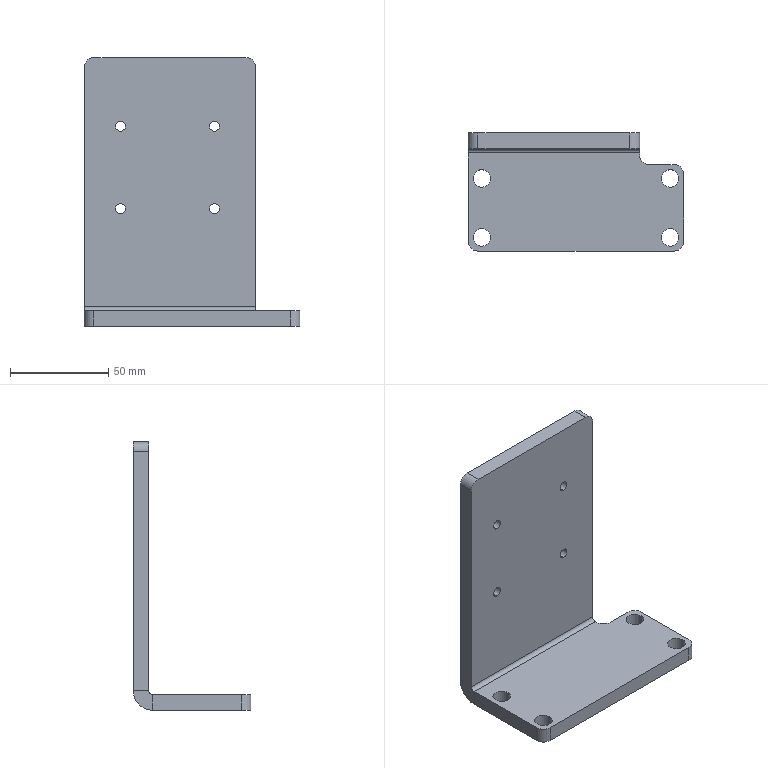Part | SolidWorks | features HoleWzd 2, EdgeFlange 1, Fillet 1, FlatPattern 1, ICE 1, SMBaseFlange 1, SheetMetal 1 | 1 solid | 38 faces | box 110 x 60 x 137 mm | volume 135582 mm3 | cylinder 24 | plane 14 | commonest cylinder face diameters 5 x8 9 x8 10 x6 4 x1 20 x1
STEP:
#1=CARTESIAN_POINT('',(107.5,7.,0.));
#2=VERTEX_POINT('',#1);
#3=CARTESIAN_POINT('',(98.5,7.,0.));
#4=VERTEX_POINT('',#3);
#5=CARTESIAN_POINT('',(103.,7.,0.));
#6=DIRECTION('',(0.,0.,-1.));
#7=DIRECTION('',(-1.,0.,0.));
#8=AXIS2_PLACEMENT_3D('',#5,#6,#7);
#9=CIRCLE('',#8,4.5);
#10=EDGE_CURVE('',#2,#4,#9,.T.);
#11=ORIENTED_EDGE('',*,*,#10,.F.);
#12=CARTESIAN_POINT('',(107.5,7.,-8.));
#13=VERTEX_POINT('',#12);
#14=CARTESIAN_POINT('',(107.5,7.,-8.));
#15=DIRECTION('',(0.,0.,-1.));
#16=VECTOR('',#15,1000.);
#17=LINE('',#14,#16);
#18=EDGE_CURVE('',#2,#13,#17,.T.);
#19=ORIENTED_EDGE('',*,*,#18,.T.);
#20=CARTESIAN_POINT('',(98.5,7.,-8.));
#21=VERTEX_POINT('',#20);
#22=CARTESIAN_POINT('',(103.,7.,-8.));
#23=DIRECTION('',(0.,0.,-1.));
#24=DIRECTION('',(-1.,0.,0.));
#25=AXIS2_PLACEMENT_3D('',#22,#23,#24);
#26=CIRCLE('',#25,4.5);
#27=EDGE_CURVE('',#13,#21,#26,.T.);
#28=ORIENTED_EDGE('',*,*,#27,.T.);
#29=CARTESIAN_POINT('',(98.5,7.,-8.));
#30=DIRECTION('',(0.,0.,-1.));
#31=VECTOR('',#30,1000.);
#32=LINE('',#29,#31);
#33=EDGE_CURVE('',#4,#21,#32,.T.);
#34=ORIENTED_EDGE('',*,*,#33,.F.);
#35=EDGE_LOOP('',(#11,#19,#28,#34));
#36=FACE_OUTER_BOUND('',#35,.T.);
#37=CARTESIAN_POINT('',(103.,7.,-8.));
#38=DIRECTION('',(0.,0.,-1.));
#39=DIRECTION('',(-1.,0.,0.));
#40=AXIS2_PLACEMENT_3D('',#37,#38,#39);
#41=CYLINDRICAL_SURFACE('',#40,4.5);
#42=ADVANCED_FACE('',(#36),#41,.F.);
#43=CARTESIAN_POINT('',(107.5,37.,0.));
#44=VERTEX_POINT('',#43);
#45=CARTESIAN_POINT('',(98.5,37.,0.));
#46=VERTEX_POINT('',#45);
#47=CARTESIAN_POINT('',(103.,37.,0.));
#48=DIRECTION('',(0.,0.,-1.));
#49=DIRECTION('',(-1.,0.,0.));
#50=AXIS2_PLACEMENT_3D('',#47,#48,#49);
#51=CIRCLE('',#50,4.5);
#52=EDGE_CURVE('',#44,#46,#51,.T.);
#53=ORIENTED_EDGE('',*,*,#52,.F.);
#54=CARTESIAN_POINT('',(107.5,37.,-8.));
#55=VERTEX_POINT('',#54);
#56=CARTESIAN_POINT('',(107.5,37.,-8.));
#57=DIRECTION('',(0.,0.,-1.));
#58=VECTOR('',#57,1000.);
#59=LINE('',#56,#58);
#60=EDGE_CURVE('',#44,#55,#59,.T.);
#61=ORIENTED_EDGE('',*,*,#60,.T.);
#62=CARTESIAN_POINT('',(98.5,37.,-8.));
#63=VERTEX_POINT('',#62);
#64=CARTESIAN_POINT('',(103.,37.,-8.));
#65=DIRECTION('',(0.,0.,-1.));
#66=DIRECTION('',(-1.,0.,0.));
#67=AXIS2_PLACEMENT_3D('',#64,#65,#66);
#68=CIRCLE('',#67,4.5);
#69=EDGE_CURVE('',#55,#63,#68,.T.);
#70=ORIENTED_EDGE('',*,*,#69,.T.);
#71=CARTESIAN_POINT('',(98.5,37.,-8.));
#72=DIRECTION('',(0.,0.,-1.));
#73=VECTOR('',#72,1000.);
#74=LINE('',#71,#73);
#75=EDGE_CURVE('',#46,#63,#74,.T.);
#76=ORIENTED_EDGE('',*,*,#75,.F.);
#77=EDGE_LOOP('',(#53,#61,#70,#76));
#78=FACE_OUTER_BOUND('',#77,.T.);
#79=CARTESIAN_POINT('',(103.,37.,-8.));
#80=DIRECTION('',(0.,0.,-1.));
#81=DIRECTION('',(-1.,0.,0.));
#82=AXIS2_PLACEMENT_3D('',#79,#80,#81);
#83=CYLINDRICAL_SURFACE('',#82,4.5);
#84=ADVANCED_FACE('',(#78),#83,.F.);
#85=CARTESIAN_POINT('',(11.5,7.,0.));
#86=VERTEX_POINT('',#85);
#87=CARTESIAN_POINT('',(2.5,7.,0.));
#88=VERTEX_POINT('',#87);
#89=CARTESIAN_POINT('',(7.,7.,0.));
#90=DIRECTION('',(0.,0.,-1.));
#91=DIRECTION('',(-1.,0.,0.));
#92=AXIS2_PLACEMENT_3D('',#89,#90,#91);
#93=CIRCLE('',#92,4.5);
#94=EDGE_CURVE('',#86,#88,#93,.T.);
#95=ORIENTED_EDGE('',*,*,#94,.F.);
#96=CARTESIAN_POINT('',(11.5,7.,-8.));
#97=VERTEX_POINT('',#96);
#98=CARTESIAN_POINT('',(11.5,7.,-8.));
#99=DIRECTION('',(0.,0.,-1.));
#100=VECTOR('',#99,1000.);
#101=LINE('',#98,#100);
#102=EDGE_CURVE('',#86,#97,#101,.T.);
#103=ORIENTED_EDGE('',*,*,#102,.T.);
#104=CARTESIAN_POINT('',(2.5,7.,-8.));
#105=VERTEX_POINT('',#104);
#106=CARTESIAN_POINT('',(7.,7.,-8.));
#107=DIRECTION('',(0.,0.,-1.));
#108=DIRECTION('',(-1.,0.,0.));
#109=AXIS2_PLACEMENT_3D('',#106,#107,#108);
#110=CIRCLE('',#109,4.5);
#111=EDGE_CURVE('',#97,#105,#110,.T.);
#112=ORIENTED_EDGE('',*,*,#111,.T.);
#113=CARTESIAN_POINT('',(2.5,7.,-8.));
#114=DIRECTION('',(0.,0.,-1.));
#115=VECTOR('',#114,1000.);
#116=LINE('',#113,#115);
#117=EDGE_CURVE('',#88,#105,#116,.T.);
#118=ORIENTED_EDGE('',*,*,#117,.F.);
#119=EDGE_LOOP('',(#95,#103,#112,#118));
#120=FACE_OUTER_BOUND('',#119,.T.);
#121=CARTESIAN_POINT('',(7.,7.,-8.));
#122=DIRECTION('',(0.,0.,-1.));
#123=DIRECTION('',(-1.,0.,0.));
#124=AXIS2_PLACEMENT_3D('',#121,#122,#123);
#125=CYLINDRICAL_SURFACE('',#124,4.5);
#126=ADVANCED_FACE('',(#120),#125,.F.);
#127=CARTESIAN_POINT('',(11.5,37.,0.));
#128=VERTEX_POINT('',#127);
#129=CARTESIAN_POINT('',(2.5,37.,0.));
#130=VERTEX_POINT('',#129);
#131=CARTESIAN_POINT('',(7.,37.,0.));
#132=DIRECTION('',(0.,0.,-1.));
#133=DIRECTION('',(-1.,0.,0.));
#134=AXIS2_PLACEMENT_3D('',#131,#132,#133);
#135=CIRCLE('',#134,4.5);
#136=EDGE_CURVE('',#128,#130,#135,.T.);
#137=ORIENTED_EDGE('',*,*,#136,.F.);
#138=CARTESIAN_POINT('',(11.5,37.,-8.));
#139=VERTEX_POINT('',#138);
#140=CARTESIAN_POINT('',(11.5,37.,-8.));
#141=DIRECTION('',(0.,0.,-1.));
#142=VECTOR('',#141,1000.);
#143=LINE('',#140,#142);
#144=EDGE_CURVE('',#128,#139,#143,.T.);
#145=ORIENTED_EDGE('',*,*,#144,.T.);
#146=CARTESIAN_POINT('',(2.5,37.,-8.));
#147=VERTEX_POINT('',#146);
#148=CARTESIAN_POINT('',(7.,37.,-8.));
#149=DIRECTION('',(0.,0.,-1.));
#150=DIRECTION('',(-1.,0.,0.));
#151=AXIS2_PLACEMENT_3D('',#148,#149,#150);
#152=CIRCLE('',#151,4.5);
#153=EDGE_CURVE('',#139,#147,#152,.T.);
#154=ORIENTED_EDGE('',*,*,#153,.T.);
#155=CARTESIAN_POINT('',(2.5,37.,-8.));
#156=DIRECTION('',(0.,0.,-1.));
#157=VECTOR('',#156,1000.);
#158=LINE('',#155,#157);
#159=EDGE_CURVE('',#130,#147,#158,.T.);
#160=ORIENTED_EDGE('',*,*,#159,.F.);
#161=EDGE_LOOP('',(#137,#145,#154,#160));
#162=FACE_OUTER_BOUND('',#161,.T.);
#163=CARTESIAN_POINT('',(7.,37.,-8.));
#164=DIRECTION('',(0.,0.,-1.));
#165=DIRECTION('',(-1.,0.,0.));
#166=AXIS2_PLACEMENT_3D('',#163,#164,#165);
#167=CYLINDRICAL_SURFACE('',#166,4.5);
#168=ADVANCED_FACE('',(#162),#167,.F.);
#169=CARTESIAN_POINT('',(18.5,52.,54.5));
#170=VERTEX_POINT('',#169);
#171=CARTESIAN_POINT('',(18.5,52.,49.5));
#172=VERTEX_POINT('',#171);
#173=CARTESIAN_POINT('',(18.5,52.,52.));
#174=DIRECTION('',(0.,-1.,0.));
#175=DIRECTION('',(0.,0.,-1.));
#176=AXIS2_PLACEMENT_3D('',#173,#174,#175);
#177=CIRCLE('',#176,2.5);
#178=EDGE_CURVE('',#170,#172,#177,.T.);
#179=ORIENTED_EDGE('',*,*,#178,.T.);
#180=CARTESIAN_POINT('',(18.5,60.,49.5));
#181=VERTEX_POINT('',#180);
#182=CARTESIAN_POINT('',(18.5,60.,49.5));
#183=DIRECTION('',(0.,1.,0.));
#184=VECTOR('',#183,1000.);
#185=LINE('',#182,#184);
#186=EDGE_CURVE('',#172,#181,#185,.T.);
#187=ORIENTED_EDGE('',*,*,#186,.T.);
#188=CARTESIAN_POINT('',(18.5,60.,54.5));
#189=VERTEX_POINT('',#188);
#190=CARTESIAN_POINT('',(18.5,60.,52.));
#191=DIRECTION('',(0.,1.,0.));
#192=DIRECTION('',(0.,0.,1.));
#193=AXIS2_PLACEMENT_3D('',#190,#191,#192);
#194=CIRCLE('',#193,2.5);
#195=EDGE_CURVE('',#181,#189,#194,.T.);
#196=ORIENTED_EDGE('',*,*,#195,.T.);
#197=CARTESIAN_POINT('',(18.5,60.,54.5));
#198=DIRECTION('',(0.,1.,0.));
#199=VECTOR('',#198,1000.);
#200=LINE('',#197,#199);
#201=EDGE_CURVE('',#170,#189,#200,.T.);
#202=ORIENTED_EDGE('',*,*,#201,.F.);
#203=EDGE_LOOP('',(#179,#187,#196,#202));
#204=FACE_OUTER_BOUND('',#203,.T.);
#205=CARTESIAN_POINT('',(18.5,60.,52.));
#206=DIRECTION('',(0.,1.,0.));
#207=DIRECTION('',(0.,0.,1.));
#208=AXIS2_PLACEMENT_3D('',#205,#206,#207);
#209=CYLINDRICAL_SURFACE('',#208,2.5);
#210=ADVANCED_FACE('',(#204),#209,.F.);
#211=CARTESIAN_POINT('',(66.5,52.,54.5));
#212=VERTEX_POINT('',#211);
#213=CARTESIAN_POINT('',(66.5,52.,49.5));
#214=VERTEX_POINT('',#213);
#215=CARTESIAN_POINT('',(66.5,52.,52.));
#216=DIRECTION('',(0.,-1.,0.));
#217=DIRECTION('',(0.,0.,-1.));
#218=AXIS2_PLACEMENT_3D('',#215,#216,#217);
#219=CIRCLE('',#218,2.5);
#220=EDGE_CURVE('',#212,#214,#219,.T.);
#221=ORIENTED_EDGE('',*,*,#220,.T.);
#222=CARTESIAN_POINT('',(66.5,60.,49.5));
#223=VERTEX_POINT('',#222);
#224=CARTESIAN_POINT('',(66.5,60.,49.5));
#225=DIRECTION('',(0.,1.,0.));
#226=VECTOR('',#225,1000.);
#227=LINE('',#224,#226);
#228=EDGE_CURVE('',#214,#223,#227,.T.);
#229=ORIENTED_EDGE('',*,*,#228,.T.);
#230=CARTESIAN_POINT('',(66.5,60.,54.5));
#231=VERTEX_POINT('',#230);
#232=CARTESIAN_POINT('',(66.5,60.,52.));
#233=DIRECTION('',(0.,1.,0.));
#234=DIRECTION('',(0.,0.,1.));
#235=AXIS2_PLACEMENT_3D('',#232,#233,#234);
#236=CIRCLE('',#235,2.5);
#237=EDGE_CURVE('',#223,#231,#236,.T.);
#238=ORIENTED_EDGE('',*,*,#237,.T.);
#239=CARTESIAN_POINT('',(66.5,60.,54.5));
#240=DIRECTION('',(0.,1.,0.));
#241=VECTOR('',#240,1000.);
#242=LINE('',#239,#241);
#243=EDGE_CURVE('',#212,#231,#242,.T.);
#244=ORIENTED_EDGE('',*,*,#243,.F.);
#245=EDGE_LOOP('',(#221,#229,#238,#244));
#246=FACE_OUTER_BOUND('',#245,.T.);
#247=CARTESIAN_POINT('',(66.5,60.,52.));
#248=DIRECTION('',(0.,1.,0.));
#249=DIRECTION('',(0.,0.,1.));
#250=AXIS2_PLACEMENT_3D('',#247,#248,#249);
#251=CYLINDRICAL_SURFACE('',#250,2.5);
#252=ADVANCED_FACE('',(#246),#251,.F.);
#253=CARTESIAN_POINT('',(18.5,52.,96.5));
#254=VERTEX_POINT('',#253);
#255=CARTESIAN_POINT('',(18.5,52.,91.5));
#256=VERTEX_POINT('',#255);
#257=CARTESIAN_POINT('',(18.5,52.,94.));
#258=DIRECTION('',(0.,-1.,0.));
#259=DIRECTION('',(0.,0.,-1.));
#260=AXIS2_PLACEMENT_3D('',#257,#258,#259);
#261=CIRCLE('',#260,2.5);
#262=EDGE_CURVE('',#254,#256,#261,.T.);
#263=ORIENTED_EDGE('',*,*,#262,.T.);
#264=CARTESIAN_POINT('',(18.5,60.,91.5));
#265=VERTEX_POINT('',#264);
#266=CARTESIAN_POINT('',(18.5,60.,91.5));
#267=DIRECTION('',(0.,1.,0.));
#268=VECTOR('',#267,1000.);
#269=LINE('',#266,#268);
#270=EDGE_CURVE('',#256,#265,#269,.T.);
#271=ORIENTED_EDGE('',*,*,#270,.T.);
#272=CARTESIAN_POINT('',(18.5,60.,96.5));
#273=VERTEX_POINT('',#272);
#274=CARTESIAN_POINT('',(18.5,60.,94.));
#275=DIRECTION('',(0.,1.,0.));
#276=DIRECTION('',(0.,0.,1.));
#277=AXIS2_PLACEMENT_3D('',#274,#275,#276);
#278=CIRCLE('',#277,2.5);
#279=EDGE_CURVE('',#265,#273,#278,.T.);
#280=ORIENTED_EDGE('',*,*,#279,.T.);
#281=CARTESIAN_POINT('',(18.5,60.,96.5));
#282=DIRECTION('',(0.,1.,0.));
#283=VECTOR('',#282,1000.);
#284=LINE('',#281,#283);
#285=EDGE_CURVE('',#254,#273,#284,.T.);
#286=ORIENTED_EDGE('',*,*,#285,.F.);
#287=EDGE_LOOP('',(#263,#271,#280,#286));
#288=FACE_OUTER_BOUND('',#287,.T.);
#289=CARTESIAN_POINT('',(18.5,60.,94.));
#290=DIRECTION('',(0.,1.,0.));
#291=DIRECTION('',(0.,0.,1.));
#292=AXIS2_PLACEMENT_3D('',#289,#290,#291);
#293=CYLINDRICAL_SURFACE('',#292,2.5);
#294=ADVANCED_FACE('',(#288),#293,.F.);
#295=CARTESIAN_POINT('',(66.5,52.,96.5));
#296=VERTEX_POINT('',#295);
#297=CARTESIAN_POINT('',(66.5,52.,91.5));
#298=VERTEX_POINT('',#297);
#299=CARTESIAN_POINT('',(66.5,52.,94.));
#300=DIRECTION('',(0.,-1.,0.));
#301=DIRECTION('',(0.,0.,-1.));
#302=AXIS2_PLACEMENT_3D('',#299,#300,#301);
#303=CIRCLE('',#302,2.5);
#304=EDGE_CURVE('',#296,#298,#303,.T.);
#305=ORIENTED_EDGE('',*,*,#304,.T.);
#306=CARTESIAN_POINT('',(66.5,60.,91.5));
#307=VERTEX_POINT('',#306);
#308=CARTESIAN_POINT('',(66.5,60.,91.5));
#309=DIRECTION('',(0.,1.,0.));
#310=VECTOR('',#309,1000.);
#311=LINE('',#308,#310);
#312=EDGE_CURVE('',#298,#307,#311,.T.);
#313=ORIENTED_EDGE('',*,*,#312,.T.);
#314=CARTESIAN_POINT('',(66.5,60.,96.5));
#315=VERTEX_POINT('',#314);
#316=CARTESIAN_POINT('',(66.5,60.,94.));
#317=DIRECTION('',(0.,1.,0.));
#318=DIRECTION('',(0.,0.,1.));
#319=AXIS2_PLACEMENT_3D('',#316,#317,#318);
#320=CIRCLE('',#319,2.5);
#321=EDGE_CURVE('',#307,#315,#320,.T.);
#322=ORIENTED_EDGE('',*,*,#321,.T.);
#323=CARTESIAN_POINT('',(66.5,60.,96.5));
#324=DIRECTION('',(0.,1.,0.));
#325=VECTOR('',#324,1000.);
#326=LINE('',#323,#325);
#327=EDGE_CURVE('',#296,#315,#326,.T.);
#328=ORIENTED_EDGE('',*,*,#327,.F.);
#329=EDGE_LOOP('',(#305,#313,#322,#328));
#330=FACE_OUTER_BOUND('',#329,.T.);
#331=CARTESIAN_POINT('',(66.5,60.,94.));
#332=DIRECTION('',(0.,1.,0.));
#333=DIRECTION('',(0.,0.,1.));
#334=AXIS2_PLACEMENT_3D('',#331,#332,#333);
#335=CYLINDRICAL_SURFACE('',#334,2.5);
#336=ADVANCED_FACE('',(#330),#335,.F.);
#337=CARTESIAN_POINT('',(87.5,60.,124.));
#338=VERTEX_POINT('',#337);
#339=CARTESIAN_POINT('',(87.5,60.,2.));
#340=VERTEX_POINT('',#339);
#341=CARTESIAN_POINT('',(87.5,60.,0.));
#342=DIRECTION('',(0.,0.,-1.));
#343=VECTOR('',#342,1000.);
#344=LINE('',#341,#343);
#345=EDGE_CURVE('',#338,#340,#344,.T.);
#346=ORIENTED_EDGE('',*,*,#345,.F.);
#347=CARTESIAN_POINT('',(87.5,52.,124.));
#348=VERTEX_POINT('',#347);
#349=CARTESIAN_POINT('',(87.5,44.,124.));
#350=DIRECTION('',(0.,-1.,0.));
#351=VECTOR('',#350,1000.);
#352=LINE('',#349,#351);
#353=EDGE_CURVE('',#338,#348,#352,.T.);
#354=ORIENTED_EDGE('',*,*,#353,.T.);
#355=CARTESIAN_POINT('',(87.5,52.,2.));
#356=VERTEX_POINT('',#355);
#357=CARTESIAN_POINT('',(87.5,52.,0.));
#358=DIRECTION('',(0.,0.,-1.));
#359=VECTOR('',#358,1000.);
#360=LINE('',#357,#359);
#361=EDGE_CURVE('',#348,#356,#360,.T.);
#362=ORIENTED_EDGE('',*,*,#361,.T.);
#363=CARTESIAN_POINT('',(87.5,52.,2.));
#364=DIRECTION('',(0.,1.,0.));
#365=VECTOR('',#364,1000.);
#366=LINE('',#363,#365);
#367=EDGE_CURVE('',#356,#340,#366,.T.);
#368=ORIENTED_EDGE('',*,*,#367,.T.);
#369=EDGE_LOOP('',(#346,#354,#362,#368));
#370=FACE_OUTER_BOUND('',#369,.T.);
#371=CARTESIAN_POINT('',(87.5,44.,129.));
#372=DIRECTION('',(-1.,0.,0.));
#373=DIRECTION('',(0.,0.,1.));
#374=AXIS2_PLACEMENT_3D('',#371,#372,#373);
#375=PLANE('',#374);
#376=ADVANCED_FACE('',(#370),#375,.F.);
#377=CARTESIAN_POINT('',(87.5,49.,0.));
#378=VERTEX_POINT('',#377);
#379=CARTESIAN_POINT('',(87.5,50.,0.));
#380=VERTEX_POINT('',#379);
#381=CARTESIAN_POINT('',(87.5,0.,0.));
#382=DIRECTION('',(0.,1.,0.));
#383=VECTOR('',#382,1000.);
#384=LINE('',#381,#383);
#385=EDGE_CURVE('',#378,#380,#384,.T.);
#386=ORIENTED_EDGE('',*,*,#385,.F.);
#387=CARTESIAN_POINT('',(87.5,49.,-8.));
#388=VERTEX_POINT('',#387);
#389=CARTESIAN_POINT('',(87.5,49.,-8.));
#390=DIRECTION('',(0.,0.,-1.));
#391=VECTOR('',#390,1000.);
#392=LINE('',#389,#391);
#393=EDGE_CURVE('',#378,#388,#392,.T.);
#394=ORIENTED_EDGE('',*,*,#393,.T.);
#395=CARTESIAN_POINT('',(87.5,50.,-8.));
#396=VERTEX_POINT('',#395);
#397=CARTESIAN_POINT('',(87.5,44.,-8.));
#398=DIRECTION('',(0.,1.,0.));
#399=VECTOR('',#398,1000.);
#400=LINE('',#397,#399);
#401=EDGE_CURVE('',#388,#396,#400,.T.);
#402=ORIENTED_EDGE('',*,*,#401,.T.);
#403=CARTESIAN_POINT('',(87.5,50.,-8.));
#404=DIRECTION('',(0.,0.,1.));
#405=VECTOR('',#404,1000.);
#406=LINE('',#403,#405);
#407=EDGE_CURVE('',#396,#380,#406,.T.);
#408=ORIENTED_EDGE('',*,*,#407,.T.);
#409=EDGE_LOOP('',(#386,#394,#402,#408));
#410=FACE_OUTER_BOUND('',#409,.T.);
#411=CARTESIAN_POINT('',(87.5,44.,129.));
#412=DIRECTION('',(-1.,0.,0.));
#413=DIRECTION('',(0.,0.,1.));
#414=AXIS2_PLACEMENT_3D('',#411,#412,#413);
#415=PLANE('',#414);
#416=ADVANCED_FACE('',(#410),#415,.F.);
#417=CARTESIAN_POINT('',(0.,50.,-8.));
#418=VERTEX_POINT('',#417);
#419=CARTESIAN_POINT('',(0.,5.,-8.));
#420=VERTEX_POINT('',#419);
#421=CARTESIAN_POINT('',(0.,0.,-8.));
#422=DIRECTION('',(0.,-1.,0.));
#423=VECTOR('',#422,1000.);
#424=LINE('',#421,#423);
#425=EDGE_CURVE('',#418,#420,#424,.T.);
#426=ORIENTED_EDGE('',*,*,#425,.T.);
#427=CARTESIAN_POINT('',(0.,5.,0.));
#428=VERTEX_POINT('',#427);
#429=CARTESIAN_POINT('',(0.,5.,-8.));
#430=DIRECTION('',(0.,0.,1.));
#431=VECTOR('',#430,1000.);
#432=LINE('',#429,#431);
#433=EDGE_CURVE('',#420,#428,#432,.T.);
#434=ORIENTED_EDGE('',*,*,#433,.T.);
#435=CARTESIAN_POINT('',(0.,50.,0.));
#436=VERTEX_POINT('',#435);
#437=CARTESIAN_POINT('',(0.,0.,0.));
#438=DIRECTION('',(0.,-1.,0.));
#439=VECTOR('',#438,1000.);
#440=LINE('',#437,#439);
#441=EDGE_CURVE('',#436,#428,#440,.T.);
#442=ORIENTED_EDGE('',*,*,#441,.F.);
#443=CARTESIAN_POINT('',(0.,50.,0.));
#444=DIRECTION('',(0.,0.,-1.));
#445=VECTOR('',#444,1000.);
#446=LINE('',#443,#445);
#447=EDGE_CURVE('',#436,#418,#446,.T.);
#448=ORIENTED_EDGE('',*,*,#447,.T.);
#449=EDGE_LOOP('',(#426,#434,#442,#448));
#450=FACE_OUTER_BOUND('',#449,.T.);
#451=CARTESIAN_POINT('',(0.,0.,-8.));
#452=DIRECTION('',(-1.,0.,0.));
#453=DIRECTION('',(0.,-1.,0.));
#454=AXIS2_PLACEMENT_3D('',#451,#452,#453);
#455=PLANE('',#454);
#456=ADVANCED_FACE('',(#450),#455,.T.);
#457=CARTESIAN_POINT('',(103.,7.,-8.));
#458=DIRECTION('',(0.,0.,-1.));
#459=DIRECTION('',(-1.,0.,0.));
#460=AXIS2_PLACEMENT_3D('',#457,#458,#459);
#461=CIRCLE('',#460,4.5);
#462=EDGE_CURVE('',#21,#13,#461,.T.);
#463=ORIENTED_EDGE('',*,*,#462,.F.);
#464=ORIENTED_EDGE('',*,*,#27,.F.);
#465=EDGE_LOOP('',(#463,#464));
#466=FACE_BOUND('',#465,.T.);
#467=CARTESIAN_POINT('',(103.,37.,-8.));
#468=DIRECTION('',(0.,0.,-1.));
#469=DIRECTION('',(-1.,0.,0.));
#470=AXIS2_PLACEMENT_3D('',#467,#468,#469);
#471=CIRCLE('',#470,4.5);
#472=EDGE_CURVE('',#63,#55,#471,.T.);
#473=ORIENTED_EDGE('',*,*,#472,.F.);
#474=ORIENTED_EDGE('',*,*,#69,.F.);
#475=EDGE_LOOP('',(#473,#474));
#476=FACE_BOUND('',#475,.T.);
#477=CARTESIAN_POINT('',(7.,7.,-8.));
#478=DIRECTION('',(0.,0.,-1.));
#479=DIRECTION('',(-1.,0.,0.));
#480=AXIS2_PLACEMENT_3D('',#477,#478,#479);
#481=CIRCLE('',#480,4.5);
#482=EDGE_CURVE('',#105,#97,#481,.T.);
#483=ORIENTED_EDGE('',*,*,#482,.F.);
#484=ORIENTED_EDGE('',*,*,#111,.F.);
#485=EDGE_LOOP('',(#483,#484));
#486=FACE_BOUND('',#485,.T.);
#487=CARTESIAN_POINT('',(7.,37.,-8.));
#488=DIRECTION('',(0.,0.,-1.));
#489=DIRECTION('',(-1.,0.,0.));
#490=AXIS2_PLACEMENT_3D('',#487,#488,#489);
#491=CIRCLE('',#490,4.5);
#492=EDGE_CURVE('',#147,#139,#491,.T.);
#493=ORIENTED_EDGE('',*,*,#492,.F.);
#494=ORIENTED_EDGE('',*,*,#153,.F.);
#495=EDGE_LOOP('',(#493,#494));
#496=FACE_BOUND('',#495,.T.);
#497=CARTESIAN_POINT('',(105.,44.,-8.));
#498=VERTEX_POINT('',#497);
#499=CARTESIAN_POINT('',(92.5,44.,-8.));
#500=VERTEX_POINT('',#499);
#501=CARTESIAN_POINT('',(110.,44.,-8.));
#502=DIRECTION('',(-1.,0.,0.));
#503=VECTOR('',#502,1000.);
#504=LINE('',#501,#503);
#505=EDGE_CURVE('',#498,#500,#504,.T.);
#506=ORIENTED_EDGE('',*,*,#505,.F.);
#507=CARTESIAN_POINT('',(110.,39.,-8.));
#508=VERTEX_POINT('',#507);
#509=CARTESIAN_POINT('',(105.,39.,-8.));
#510=DIRECTION('',(0.,0.,-1.));
#511=DIRECTION('',(-1.,0.,0.));
#512=AXIS2_PLACEMENT_3D('',#509,#510,#511);
#513=CIRCLE('',#512,5.);
#514=EDGE_CURVE('',#498,#508,#513,.T.);
#515=ORIENTED_EDGE('',*,*,#514,.T.);
#516=CARTESIAN_POINT('',(110.,5.,-8.));
#517=VERTEX_POINT('',#516);
#518=CARTESIAN_POINT('',(110.,0.,-8.));
#519=DIRECTION('',(0.,1.,0.));
#520=VECTOR('',#519,1000.);
#521=LINE('',#518,#520);
#522=EDGE_CURVE('',#517,#508,#521,.T.);
#523=ORIENTED_EDGE('',*,*,#522,.F.);
#524=CARTESIAN_POINT('',(105.,0.,-8.));
#525=VERTEX_POINT('',#524);
#526=CARTESIAN_POINT('',(105.,5.,-8.));
#527=DIRECTION('',(0.,0.,-1.));
#528=DIRECTION('',(-1.,0.,0.));
#529=AXIS2_PLACEMENT_3D('',#526,#527,#528);
#530=CIRCLE('',#529,5.);
#531=EDGE_CURVE('',#517,#525,#530,.T.);
#532=ORIENTED_EDGE('',*,*,#531,.T.);
#533=CARTESIAN_POINT('',(5.,0.,-8.));
#534=VERTEX_POINT('',#533);
#535=CARTESIAN_POINT('',(0.,0.,-8.));
#536=DIRECTION('',(1.,0.,0.));
#537=VECTOR('',#536,1000.);
#538=LINE('',#535,#537);
#539=EDGE_CURVE('',#534,#525,#538,.T.);
#540=ORIENTED_EDGE('',*,*,#539,.F.);
#541=CARTESIAN_POINT('',(5.,5.,-8.));
#542=DIRECTION('',(0.,0.,-1.));
#543=DIRECTION('',(-1.,0.,0.));
#544=AXIS2_PLACEMENT_3D('',#541,#542,#543);
#545=CIRCLE('',#544,5.);
#546=EDGE_CURVE('',#534,#420,#545,.T.);
#547=ORIENTED_EDGE('',*,*,#546,.T.);
#548=ORIENTED_EDGE('',*,*,#425,.F.);
#549=CARTESIAN_POINT('',(0.,50.,-8.));
#550=DIRECTION('',(1.,0.,0.));
#551=VECTOR('',#550,1000.);
#552=LINE('',#549,#551);
#553=EDGE_CURVE('',#418,#396,#552,.T.);
#554=ORIENTED_EDGE('',*,*,#553,.T.);
#555=ORIENTED_EDGE('',*,*,#401,.F.);
#556=CARTESIAN_POINT('',(92.5,49.,-8.));
#557=DIRECTION('',(0.,0.,1.));
#558=DIRECTION('',(-1.,0.,0.));
#559=AXIS2_PLACEMENT_3D('',#556,#557,#558);
#560=CIRCLE('',#559,5.);
#561=EDGE_CURVE('',#388,#500,#560,.T.);
#562=ORIENTED_EDGE('',*,*,#561,.T.);
#563=EDGE_LOOP('',(#506,#515,#523,#532,#540,#547,#548,#554,#555,#562));
#564=FACE_OUTER_BOUND('',#563,.T.);
#565=CARTESIAN_POINT('',(0.,0.,-8.));
#566=DIRECTION('',(0.,0.,-1.));
#567=DIRECTION('',(-1.,0.,0.));
#568=AXIS2_PLACEMENT_3D('',#565,#566,#567);
#569=PLANE('',#568);
#570=ADVANCED_FACE('',(#466,#476,#486,#496,#564),#569,.T.);
#571=CARTESIAN_POINT('',(103.,7.,0.));
#572=DIRECTION('',(0.,0.,-1.));
#573=DIRECTION('',(-1.,0.,0.));
#574=AXIS2_PLACEMENT_3D('',#571,#572,#573);
#575=CIRCLE('',#574,4.5);
#576=EDGE_CURVE('',#4,#2,#575,.T.);
#577=ORIENTED_EDGE('',*,*,#576,.T.);
#578=ORIENTED_EDGE('',*,*,#10,.T.);
#579=EDGE_LOOP('',(#577,#578));
#580=FACE_BOUND('',#579,.T.);
#581=CARTESIAN_POINT('',(103.,37.,0.));
#582=DIRECTION('',(0.,0.,-1.));
#583=DIRECTION('',(-1.,0.,0.));
#584=AXIS2_PLACEMENT_3D('',#581,#582,#583);
#585=CIRCLE('',#584,4.5);
#586=EDGE_CURVE('',#46,#44,#585,.T.);
#587=ORIENTED_EDGE('',*,*,#586,.T.);
#588=ORIENTED_EDGE('',*,*,#52,.T.);
#589=EDGE_LOOP('',(#587,#588));
#590=FACE_BOUND('',#589,.T.);
#591=CARTESIAN_POINT('',(7.,7.,0.));
#592=DIRECTION('',(0.,0.,-1.));
#593=DIRECTION('',(-1.,0.,0.));
#594=AXIS2_PLACEMENT_3D('',#591,#592,#593);
#595=CIRCLE('',#594,4.5);
#596=EDGE_CURVE('',#88,#86,#595,.T.);
#597=ORIENTED_EDGE('',*,*,#596,.T.);
#598=ORIENTED_EDGE('',*,*,#94,.T.);
#599=EDGE_LOOP('',(#597,#598));
#600=FACE_BOUND('',#599,.T.);
#601=CARTESIAN_POINT('',(7.,37.,0.));
#602=DIRECTION('',(0.,0.,-1.));
#603=DIRECTION('',(-1.,0.,0.));
#604=AXIS2_PLACEMENT_3D('',#601,#602,#603);
#605=CIRCLE('',#604,4.5);
#606=EDGE_CURVE('',#130,#128,#605,.T.);
#607=ORIENTED_EDGE('',*,*,#606,.T.);
#608=ORIENTED_EDGE('',*,*,#136,.T.);
#609=EDGE_LOOP('',(#607,#608));
#610=FACE_BOUND('',#609,.T.);
#611=CARTESIAN_POINT('',(110.,5.,0.));
#612=VERTEX_POINT('',#611);
#613=CARTESIAN_POINT('',(110.,39.,0.));
#614=VERTEX_POINT('',#613);
#615=CARTESIAN_POINT('',(110.,0.,0.));
#616=DIRECTION('',(0.,1.,0.));
#617=VECTOR('',#616,1000.);
#618=LINE('',#615,#617);
#619=EDGE_CURVE('',#612,#614,#618,.T.);
#620=ORIENTED_EDGE('',*,*,#619,.T.);
#621=CARTESIAN_POINT('',(105.,44.,0.));
#622=VERTEX_POINT('',#621);
#623=CARTESIAN_POINT('',(105.,39.,0.));
#624=DIRECTION('',(0.,0.,1.));
#625=DIRECTION('',(-1.,0.,0.));
#626=AXIS2_PLACEMENT_3D('',#623,#624,#625);
#627=CIRCLE('',#626,5.);
#628=EDGE_CURVE('',#614,#622,#627,.T.);
#629=ORIENTED_EDGE('',*,*,#628,.T.);
#630=CARTESIAN_POINT('',(92.5,44.,0.));
#631=VERTEX_POINT('',#630);
#632=CARTESIAN_POINT('',(0.,44.,0.));
#633=DIRECTION('',(-1.,0.,0.));
#634=VECTOR('',#633,1000.);
#635=LINE('',#632,#634);
#636=EDGE_CURVE('',#622,#631,#635,.T.);
#637=ORIENTED_EDGE('',*,*,#636,.T.);
#638=CARTESIAN_POINT('',(92.5,49.,0.));
#639=DIRECTION('',(0.,0.,-1.));
#640=DIRECTION('',(-1.,0.,0.));
#641=AXIS2_PLACEMENT_3D('',#638,#639,#640);
#642=CIRCLE('',#641,5.);
#643=EDGE_CURVE('',#631,#378,#642,.T.);
#644=ORIENTED_EDGE('',*,*,#643,.T.);
#645=ORIENTED_EDGE('',*,*,#385,.T.);
#646=CARTESIAN_POINT('',(0.,50.,0.));
#647=DIRECTION('',(1.,0.,0.));
#648=VECTOR('',#647,1000.);
#649=LINE('',#646,#648);
#650=EDGE_CURVE('',#436,#380,#649,.T.);
#651=ORIENTED_EDGE('',*,*,#650,.F.);
#652=ORIENTED_EDGE('',*,*,#441,.T.);
#653=CARTESIAN_POINT('',(5.,0.,0.));
#654=VERTEX_POINT('',#653);
#655=CARTESIAN_POINT('',(5.,5.,0.));
#656=DIRECTION('',(0.,0.,1.));
#657=DIRECTION('',(-1.,0.,0.));
#658=AXIS2_PLACEMENT_3D('',#655,#656,#657);
#659=CIRCLE('',#658,5.);
#660=EDGE_CURVE('',#428,#654,#659,.T.);
#661=ORIENTED_EDGE('',*,*,#660,.T.);
#662=CARTESIAN_POINT('',(105.,0.,0.));
#663=VERTEX_POINT('',#662);
#664=CARTESIAN_POINT('',(0.,0.,0.));
#665=DIRECTION('',(1.,0.,0.));
#666=VECTOR('',#665,1000.);
#667=LINE('',#664,#666);
#668=EDGE_CURVE('',#654,#663,#667,.T.);
#669=ORIENTED_EDGE('',*,*,#668,.T.);
#670=CARTESIAN_POINT('',(105.,5.,0.));
#671=DIRECTION('',(0.,0.,1.));
#672=DIRECTION('',(-1.,0.,0.));
#673=AXIS2_PLACEMENT_3D('',#670,#671,#672);
#674=CIRCLE('',#673,5.);
#675=EDGE_CURVE('',#663,#612,#674,.T.);
#676=ORIENTED_EDGE('',*,*,#675,.T.);
#677=EDGE_LOOP('',(#620,#629,#637,#644,#645,#651,#652,#661,#669,#676));
#678=FACE_OUTER_BOUND('',#677,.T.);
#679=CARTESIAN_POINT('',(0.,0.,0.));
#680=DIRECTION('',(0.,0.,-1.));
#681=DIRECTION('',(-1.,0.,0.));
#682=AXIS2_PLACEMENT_3D('',#679,#680,#681);
#683=PLANE('',#682);
#684=ADVANCED_FACE('',(#580,#590,#600,#610,#678),#683,.F.);
#685=ORIENTED_EDGE('',*,*,#522,.T.);
#686=CARTESIAN_POINT('',(110.,39.,0.));
#687=DIRECTION('',(0.,0.,1.));
#688=VECTOR('',#687,1000.);
#689=LINE('',#686,#688);
#690=EDGE_CURVE('',#508,#614,#689,.T.);
#691=ORIENTED_EDGE('',*,*,#690,.T.);
#692=ORIENTED_EDGE('',*,*,#619,.F.);
#693=CARTESIAN_POINT('',(110.,5.,-8.));
#694=DIRECTION('',(0.,0.,-1.));
#695=VECTOR('',#694,1000.);
#696=LINE('',#693,#695);
#697=EDGE_CURVE('',#612,#517,#696,.T.);
#698=ORIENTED_EDGE('',*,*,#697,.T.);
#699=EDGE_LOOP('',(#685,#691,#692,#698));
#700=FACE_OUTER_BOUND('',#699,.T.);
#701=CARTESIAN_POINT('',(110.,0.,-8.));
#702=DIRECTION('',(1.,0.,0.));
#703=DIRECTION('',(0.,1.,0.));
#704=AXIS2_PLACEMENT_3D('',#701,#702,#703);
#705=PLANE('',#704);
#706=ADVANCED_FACE('',(#700),#705,.T.);
#707=ORIENTED_EDGE('',*,*,#539,.T.);
#708=CARTESIAN_POINT('',(105.,0.,-8.));
#709=DIRECTION('',(0.,0.,1.));
#710=VECTOR('',#709,1000.);
#711=LINE('',#708,#710);
#712=EDGE_CURVE('',#525,#663,#711,.T.);
#713=ORIENTED_EDGE('',*,*,#712,.T.);
#714=ORIENTED_EDGE('',*,*,#668,.F.);
#715=CARTESIAN_POINT('',(5.,0.,-8.));
#716=DIRECTION('',(0.,0.,-1.));
#717=VECTOR('',#716,1000.);
#718=LINE('',#715,#717);
#719=EDGE_CURVE('',#654,#534,#718,.T.);
#720=ORIENTED_EDGE('',*,*,#719,.T.);
#721=EDGE_LOOP('',(#707,#713,#714,#720));
#722=FACE_OUTER_BOUND('',#721,.T.);
#723=CARTESIAN_POINT('',(0.,0.,-8.));
#724=DIRECTION('',(0.,-1.,0.));
#725=DIRECTION('',(0.,0.,-1.));
#726=AXIS2_PLACEMENT_3D('',#723,#724,#725);
#727=PLANE('',#726);
#728=ADVANCED_FACE('',(#722),#727,.T.);
#729=CARTESIAN_POINT('',(0.,52.,2.));
#730=VERTEX_POINT('',#729);
#731=CARTESIAN_POINT('',(0.,50.,2.));
#732=DIRECTION('',(-1.,0.,0.));
#733=DIRECTION('',(0.,0.,1.));
#734=AXIS2_PLACEMENT_3D('',#731,#732,#733);
#735=CIRCLE('',#734,2.);
#736=EDGE_CURVE('',#730,#436,#735,.T.);
#737=ORIENTED_EDGE('',*,*,#736,.F.);
#738=CARTESIAN_POINT('',(0.,60.,2.));
#739=VERTEX_POINT('',#738);
#740=CARTESIAN_POINT('',(0.,52.,2.));
#741=DIRECTION('',(0.,1.,0.));
#742=VECTOR('',#741,1000.);
#743=LINE('',#740,#742);
#744=EDGE_CURVE('',#730,#739,#743,.T.);
#745=ORIENTED_EDGE('',*,*,#744,.T.);
#746=CARTESIAN_POINT('',(0.,50.,2.));
#747=DIRECTION('',(-1.,0.,0.));
#748=DIRECTION('',(0.,0.,1.));
#749=AXIS2_PLACEMENT_3D('',#746,#747,#748);
#750=CIRCLE('',#749,10.);
#751=EDGE_CURVE('',#739,#418,#750,.T.);
#752=ORIENTED_EDGE('',*,*,#751,.T.);
#753=ORIENTED_EDGE('',*,*,#447,.F.);
#754=EDGE_LOOP('',(#737,#745,#752,#753));
#755=FACE_OUTER_BOUND('',#754,.T.);
#756=CARTESIAN_POINT('',(0.,50.,2.));
#757=DIRECTION('',(1.,0.,0.));
#758=DIRECTION('',(0.,0.,-1.));
#759=AXIS2_PLACEMENT_3D('',#756,#757,#758);
#760=PLANE('',#759);
#761=ADVANCED_FACE('',(#755),#760,.F.);
#762=CARTESIAN_POINT('',(87.5,50.,2.));
#763=DIRECTION('',(1.,0.,0.));
#764=DIRECTION('',(0.,0.,1.));
#765=AXIS2_PLACEMENT_3D('',#762,#763,#764);
#766=CIRCLE('',#765,10.);
#767=EDGE_CURVE('',#396,#340,#766,.T.);
#768=ORIENTED_EDGE('',*,*,#767,.F.);
#769=ORIENTED_EDGE('',*,*,#553,.F.);
#770=ORIENTED_EDGE('',*,*,#751,.F.);
#771=CARTESIAN_POINT('',(110.,60.,2.));
#772=DIRECTION('',(1.,0.,0.));
#773=VECTOR('',#772,1000.);
#774=LINE('',#771,#773);
#775=EDGE_CURVE('',#739,#340,#774,.T.);
#776=ORIENTED_EDGE('',*,*,#775,.T.);
#777=EDGE_LOOP('',(#768,#769,#770,#776));
#778=FACE_OUTER_BOUND('',#777,.T.);
#779=CARTESIAN_POINT('',(0.,50.,2.));
#780=DIRECTION('',(-1.,0.,0.));
#781=DIRECTION('',(0.,1.,0.));
#782=AXIS2_PLACEMENT_3D('',#779,#780,#781);
#783=CYLINDRICAL_SURFACE('',#782,10.);
#784=ADVANCED_FACE('',(#778),#783,.T.);
#785=ORIENTED_EDGE('',*,*,#650,.T.);
#786=CARTESIAN_POINT('',(87.5,50.,2.));
#787=DIRECTION('',(1.,0.,0.));
#788=DIRECTION('',(0.,0.,1.));
#789=AXIS2_PLACEMENT_3D('',#786,#787,#788);
#790=CIRCLE('',#789,2.);
#791=EDGE_CURVE('',#380,#356,#790,.T.);
#792=ORIENTED_EDGE('',*,*,#791,.T.);
#793=CARTESIAN_POINT('',(110.,52.,2.));
#794=DIRECTION('',(-1.,0.,0.));
#795=VECTOR('',#794,1000.);
#796=LINE('',#793,#795);
#797=EDGE_CURVE('',#356,#730,#796,.T.);
#798=ORIENTED_EDGE('',*,*,#797,.T.);
#799=ORIENTED_EDGE('',*,*,#736,.T.);
#800=EDGE_LOOP('',(#785,#792,#798,#799));
#801=FACE_OUTER_BOUND('',#800,.T.);
#802=CARTESIAN_POINT('',(0.,50.,2.));
#803=DIRECTION('',(-1.,0.,0.));
#804=DIRECTION('',(0.,1.,0.));
#805=AXIS2_PLACEMENT_3D('',#802,#803,#804);
#806=CYLINDRICAL_SURFACE('',#805,2.);
#807=ADVANCED_FACE('',(#801),#806,.F.);
#808=CARTESIAN_POINT('',(0.,52.,124.));
#809=VERTEX_POINT('',#808);
#810=CARTESIAN_POINT('',(0.,52.,129.));
#811=DIRECTION('',(0.,0.,1.));
#812=VECTOR('',#811,1000.);
#813=LINE('',#810,#812);
#814=EDGE_CURVE('',#730,#809,#813,.T.);
#815=ORIENTED_EDGE('',*,*,#814,.T.);
#816=CARTESIAN_POINT('',(0.,60.,124.));
#817=VERTEX_POINT('',#816);
#818=CARTESIAN_POINT('',(0.,60.,124.));
#819=DIRECTION('',(0.,1.,0.));
#820=VECTOR('',#819,1000.);
#821=LINE('',#818,#820);
#822=EDGE_CURVE('',#809,#817,#821,.T.);
#823=ORIENTED_EDGE('',*,*,#822,.T.);
#824=CARTESIAN_POINT('',(0.,60.,0.));
#825=DIRECTION('',(0.,0.,1.));
#826=VECTOR('',#825,1000.);
#827=LINE('',#824,#826);
#828=EDGE_CURVE('',#739,#817,#827,.T.);
#829=ORIENTED_EDGE('',*,*,#828,.F.);
#830=ORIENTED_EDGE('',*,*,#744,.F.);
#831=EDGE_LOOP('',(#815,#823,#829,#830));
#832=FACE_OUTER_BOUND('',#831,.T.);
#833=CARTESIAN_POINT('',(0.,60.,129.));
#834=DIRECTION('',(1.,0.,0.));
#835=DIRECTION('',(0.,0.,-1.));
#836=AXIS2_PLACEMENT_3D('',#833,#834,#835);
#837=PLANE('',#836);
#838=ADVANCED_FACE('',(#832),#837,.F.);
#839=CARTESIAN_POINT('',(18.5,60.,52.));
#840=DIRECTION('',(0.,1.,0.));
#841=DIRECTION('',(0.,0.,1.));
#842=AXIS2_PLACEMENT_3D('',#839,#840,#841);
#843=CIRCLE('',#842,2.5);
#844=EDGE_CURVE('',#189,#181,#843,.T.);
#845=ORIENTED_EDGE('',*,*,#844,.F.);
#846=ORIENTED_EDGE('',*,*,#195,.F.);
#847=EDGE_LOOP('',(#845,#846));
#848=FACE_BOUND('',#847,.T.);
#849=CARTESIAN_POINT('',(66.5,60.,52.));
#850=DIRECTION('',(0.,1.,0.));
#851=DIRECTION('',(0.,0.,1.));
#852=AXIS2_PLACEMENT_3D('',#849,#850,#851);
#853=CIRCLE('',#852,2.5);
#854=EDGE_CURVE('',#231,#223,#853,.T.);
#855=ORIENTED_EDGE('',*,*,#854,.F.);
#856=ORIENTED_EDGE('',*,*,#237,.F.);
#857=EDGE_LOOP('',(#855,#856));
#858=FACE_BOUND('',#857,.T.);
#859=CARTESIAN_POINT('',(18.5,60.,94.));
#860=DIRECTION('',(0.,1.,0.));
#861=DIRECTION('',(0.,0.,1.));
#862=AXIS2_PLACEMENT_3D('',#859,#860,#861);
#863=CIRCLE('',#862,2.5);
#864=EDGE_CURVE('',#273,#265,#863,.T.);
#865=ORIENTED_EDGE('',*,*,#864,.F.);
#866=ORIENTED_EDGE('',*,*,#279,.F.);
#867=EDGE_LOOP('',(#865,#866));
#868=FACE_BOUND('',#867,.T.);
#869=CARTESIAN_POINT('',(66.5,60.,94.));
#870=DIRECTION('',(0.,1.,0.));
#871=DIRECTION('',(0.,0.,1.));
#872=AXIS2_PLACEMENT_3D('',#869,#870,#871);
#873=CIRCLE('',#872,2.5);
#874=EDGE_CURVE('',#315,#307,#873,.T.);
#875=ORIENTED_EDGE('',*,*,#874,.F.);
#876=ORIENTED_EDGE('',*,*,#321,.F.);
#877=EDGE_LOOP('',(#875,#876));
#878=FACE_BOUND('',#877,.T.);
#879=CARTESIAN_POINT('',(5.,60.,129.));
#880=VERTEX_POINT('',#879);
#881=CARTESIAN_POINT('',(82.5,60.,129.));
#882=VERTEX_POINT('',#881);
#883=CARTESIAN_POINT('',(0.,60.,129.));
#884=DIRECTION('',(1.,0.,0.));
#885=VECTOR('',#884,1000.);
#886=LINE('',#883,#885);
#887=EDGE_CURVE('',#880,#882,#886,.T.);
#888=ORIENTED_EDGE('',*,*,#887,.T.);
#889=CARTESIAN_POINT('',(82.5,60.,124.));
#890=DIRECTION('',(0.,1.,0.));
#891=DIRECTION('',(0.,0.,-1.));
#892=AXIS2_PLACEMENT_3D('',#889,#890,#891);
#893=CIRCLE('',#892,5.);
#894=EDGE_CURVE('',#882,#338,#893,.T.);
#895=ORIENTED_EDGE('',*,*,#894,.T.);
#896=ORIENTED_EDGE('',*,*,#345,.T.);
#897=ORIENTED_EDGE('',*,*,#775,.F.);
#898=ORIENTED_EDGE('',*,*,#828,.T.);
#899=CARTESIAN_POINT('',(5.,60.,124.));
#900=DIRECTION('',(0.,1.,0.));
#901=DIRECTION('',(0.,0.,-1.));
#902=AXIS2_PLACEMENT_3D('',#899,#900,#901);
#903=CIRCLE('',#902,5.);
#904=EDGE_CURVE('',#817,#880,#903,.T.);
#905=ORIENTED_EDGE('',*,*,#904,.T.);
#906=EDGE_LOOP('',(#888,#895,#896,#897,#898,#905));
#907=FACE_OUTER_BOUND('',#906,.T.);
#908=CARTESIAN_POINT('',(0.,60.,0.));
#909=DIRECTION('',(0.,-1.,0.));
#910=DIRECTION('',(0.,0.,-1.));
#911=AXIS2_PLACEMENT_3D('',#908,#909,#910);
#912=PLANE('',#911);
#913=ADVANCED_FACE('',(#848,#858,#868,#878,#907),#912,.F.);
#914=ORIENTED_EDGE('',*,*,#178,.F.);
#915=CARTESIAN_POINT('',(18.5,52.,52.));
#916=DIRECTION('',(0.,-1.,0.));
#917=DIRECTION('',(0.,0.,-1.));
#918=AXIS2_PLACEMENT_3D('',#915,#916,#917);
#919=CIRCLE('',#918,2.5);
#920=EDGE_CURVE('',#172,#170,#919,.T.);
#921=ORIENTED_EDGE('',*,*,#920,.F.);
#922=EDGE_LOOP('',(#914,#921));
#923=FACE_BOUND('',#922,.T.);
#924=ORIENTED_EDGE('',*,*,#220,.F.);
#925=CARTESIAN_POINT('',(66.5,52.,52.));
#926=DIRECTION('',(0.,-1.,0.));
#927=DIRECTION('',(0.,0.,-1.));
#928=AXIS2_PLACEMENT_3D('',#925,#926,#927);
#929=CIRCLE('',#928,2.5);
#930=EDGE_CURVE('',#214,#212,#929,.T.);
#931=ORIENTED_EDGE('',*,*,#930,.F.);
#932=EDGE_LOOP('',(#924,#931));
#933=FACE_BOUND('',#932,.T.);
#934=ORIENTED_EDGE('',*,*,#262,.F.);
#935=CARTESIAN_POINT('',(18.5,52.,94.));
#936=DIRECTION('',(0.,-1.,0.));
#937=DIRECTION('',(0.,0.,-1.));
#938=AXIS2_PLACEMENT_3D('',#935,#936,#937);
#939=CIRCLE('',#938,2.5);
#940=EDGE_CURVE('',#256,#254,#939,.T.);
#941=ORIENTED_EDGE('',*,*,#940,.F.);
#942=EDGE_LOOP('',(#934,#941));
#943=FACE_BOUND('',#942,.T.);
#944=ORIENTED_EDGE('',*,*,#304,.F.);
#945=CARTESIAN_POINT('',(66.5,52.,94.));
#946=DIRECTION('',(0.,-1.,0.));
#947=DIRECTION('',(0.,0.,-1.));
#948=AXIS2_PLACEMENT_3D('',#945,#946,#947);
#949=CIRCLE('',#948,2.5);
#950=EDGE_CURVE('',#298,#296,#949,.T.);
#951=ORIENTED_EDGE('',*,*,#950,.F.);
#952=EDGE_LOOP('',(#944,#951));
#953=FACE_BOUND('',#952,.T.);
#954=ORIENTED_EDGE('',*,*,#361,.F.);
#955=CARTESIAN_POINT('',(82.5,52.,129.));
#956=VERTEX_POINT('',#955);
#957=CARTESIAN_POINT('',(82.5,52.,124.));
#958=DIRECTION('',(0.,-1.,0.));
#959=DIRECTION('',(0.,0.,-1.));
#960=AXIS2_PLACEMENT_3D('',#957,#958,#959);
#961=CIRCLE('',#960,5.);
#962=EDGE_CURVE('',#348,#956,#961,.T.);
#963=ORIENTED_EDGE('',*,*,#962,.T.);
#964=CARTESIAN_POINT('',(5.,52.,129.));
#965=VERTEX_POINT('',#964);
#966=CARTESIAN_POINT('',(110.,52.,129.));
#967=DIRECTION('',(1.,0.,0.));
#968=VECTOR('',#967,1000.);
#969=LINE('',#966,#968);
#970=EDGE_CURVE('',#965,#956,#969,.T.);
#971=ORIENTED_EDGE('',*,*,#970,.F.);
#972=CARTESIAN_POINT('',(5.,52.,124.));
#973=DIRECTION('',(0.,-1.,0.));
#974=DIRECTION('',(0.,0.,-1.));
#975=AXIS2_PLACEMENT_3D('',#972,#973,#974);
#976=CIRCLE('',#975,5.);
#977=EDGE_CURVE('',#965,#809,#976,.T.);
#978=ORIENTED_EDGE('',*,*,#977,.T.);
#979=ORIENTED_EDGE('',*,*,#814,.F.);
#980=ORIENTED_EDGE('',*,*,#797,.F.);
#981=EDGE_LOOP('',(#954,#963,#971,#978,#979,#980));
#982=FACE_OUTER_BOUND('',#981,.T.);
#983=CARTESIAN_POINT('',(0.,52.,0.));
#984=DIRECTION('',(0.,-1.,0.));
#985=DIRECTION('',(0.,0.,-1.));
#986=AXIS2_PLACEMENT_3D('',#983,#984,#985);
#987=PLANE('',#986);
#988=ADVANCED_FACE('',(#923,#933,#943,#953,#982),#987,.T.);
#989=ORIENTED_EDGE('',*,*,#970,.T.);
#990=CARTESIAN_POINT('',(82.5,60.,129.));
#991=DIRECTION('',(0.,1.,0.));
#992=VECTOR('',#991,1000.);
#993=LINE('',#990,#992);
#994=EDGE_CURVE('',#956,#882,#993,.T.);
#995=ORIENTED_EDGE('',*,*,#994,.T.);
#996=ORIENTED_EDGE('',*,*,#887,.F.);
#997=CARTESIAN_POINT('',(5.,60.,129.));
#998=DIRECTION('',(0.,-1.,0.));
#999=VECTOR('',#998,1000.);
#1000=LINE('',#997,#999);
#1001=EDGE_CURVE('',#880,#965,#1000,.T.);
#1002=ORIENTED_EDGE('',*,*,#1001,.T.);
#1003=EDGE_LOOP('',(#989,#995,#996,#1002));
#1004=FACE_OUTER_BOUND('',#1003,.T.);
#1005=CARTESIAN_POINT('',(110.,60.,129.));
#1006=DIRECTION('',(0.,0.,-1.));
#1007=DIRECTION('',(0.,1.,0.));
#1008=AXIS2_PLACEMENT_3D('',#1005,#1006,#1007);
#1009=PLANE('',#1008);
#1010=ADVANCED_FACE('',(#1004),#1009,.F.);
#1011=ORIENTED_EDGE('',*,*,#505,.T.);
#1012=CARTESIAN_POINT('',(92.5,44.,0.));
#1013=DIRECTION('',(0.,0.,1.));
#1014=VECTOR('',#1013,1000.);
#1015=LINE('',#1012,#1014);
#1016=EDGE_CURVE('',#500,#631,#1015,.T.);
#1017=ORIENTED_EDGE('',*,*,#1016,.T.);
#1018=ORIENTED_EDGE('',*,*,#636,.F.);
#1019=CARTESIAN_POINT('',(105.,44.,-8.));
#1020=DIRECTION('',(0.,0.,-1.));
#1021=VECTOR('',#1020,1000.);
#1022=LINE('',#1019,#1021);
#1023=EDGE_CURVE('',#622,#498,#1022,.T.);
#1024=ORIENTED_EDGE('',*,*,#1023,.T.);
#1025=EDGE_LOOP('',(#1011,#1017,#1018,#1024));
#1026=FACE_OUTER_BOUND('',#1025,.T.);
#1027=CARTESIAN_POINT('',(110.,44.,129.));
#1028=DIRECTION('',(0.,-1.,0.));
#1029=DIRECTION('',(0.,0.,-1.));
#1030=AXIS2_PLACEMENT_3D('',#1027,#1028,#1029);
#1031=PLANE('',#1030);
#1032=ADVANCED_FACE('',(#1026),#1031,.F.);
#1033=ORIENTED_EDGE('',*,*,#367,.F.);
#1034=ORIENTED_EDGE('',*,*,#791,.F.);
#1035=ORIENTED_EDGE('',*,*,#407,.F.);
#1036=ORIENTED_EDGE('',*,*,#767,.T.);
#1037=EDGE_LOOP('',(#1033,#1034,#1035,#1036));
#1038=FACE_OUTER_BOUND('',#1037,.T.);
#1039=CARTESIAN_POINT('',(87.5,44.,129.));
#1040=DIRECTION('',(-1.,0.,0.));
#1041=DIRECTION('',(0.,0.,1.));
#1042=AXIS2_PLACEMENT_3D('',#1039,#1040,#1041);
#1043=PLANE('',#1042);
#1044=ADVANCED_FACE('',(#1038),#1043,.F.);
#1045=ORIENTED_EDGE('',*,*,#312,.F.);
#1046=ORIENTED_EDGE('',*,*,#950,.T.);
#1047=ORIENTED_EDGE('',*,*,#327,.T.);
#1048=ORIENTED_EDGE('',*,*,#874,.T.);
#1049=EDGE_LOOP('',(#1045,#1046,#1047,#1048));
#1050=FACE_OUTER_BOUND('',#1049,.T.);
#1051=CARTESIAN_POINT('',(66.5,60.,94.));
#1052=DIRECTION('',(0.,1.,0.));
#1053=DIRECTION('',(0.,0.,1.));
#1054=AXIS2_PLACEMENT_3D('',#1051,#1052,#1053);
#1055=CYLINDRICAL_SURFACE('',#1054,2.5);
#1056=ADVANCED_FACE('',(#1050),#1055,.F.);
#1057=ORIENTED_EDGE('',*,*,#270,.F.);
#1058=ORIENTED_EDGE('',*,*,#940,.T.);
#1059=ORIENTED_EDGE('',*,*,#285,.T.);
#1060=ORIENTED_EDGE('',*,*,#864,.T.);
#1061=EDGE_LOOP('',(#1057,#1058,#1059,#1060));
#1062=FACE_OUTER_BOUND('',#1061,.T.);
#1063=CARTESIAN_POINT('',(18.5,60.,94.));
#1064=DIRECTION('',(0.,1.,0.));
#1065=DIRECTION('',(0.,0.,1.));
#1066=AXIS2_PLACEMENT_3D('',#1063,#1064,#1065);
#1067=CYLINDRICAL_SURFACE('',#1066,2.5);
#1068=ADVANCED_FACE('',(#1062),#1067,.F.);
#1069=ORIENTED_EDGE('',*,*,#228,.F.);
#1070=ORIENTED_EDGE('',*,*,#930,.T.);
#1071=ORIENTED_EDGE('',*,*,#243,.T.);
#1072=ORIENTED_EDGE('',*,*,#854,.T.);
#1073=EDGE_LOOP('',(#1069,#1070,#1071,#1072));
#1074=FACE_OUTER_BOUND('',#1073,.T.);
#1075=CARTESIAN_POINT('',(66.5,60.,52.));
#1076=DIRECTION('',(0.,1.,0.));
#1077=DIRECTION('',(0.,0.,1.));
#1078=AXIS2_PLACEMENT_3D('',#1075,#1076,#1077);
#1079=CYLINDRICAL_SURFACE('',#1078,2.5);
#1080=ADVANCED_FACE('',(#1074),#1079,.F.);
#1081=ORIENTED_EDGE('',*,*,#186,.F.);
#1082=ORIENTED_EDGE('',*,*,#920,.T.);
#1083=ORIENTED_EDGE('',*,*,#201,.T.);
#1084=ORIENTED_EDGE('',*,*,#844,.T.);
#1085=EDGE_LOOP('',(#1081,#1082,#1083,#1084));
#1086=FACE_OUTER_BOUND('',#1085,.T.);
#1087=CARTESIAN_POINT('',(18.5,60.,52.));
#1088=DIRECTION('',(0.,1.,0.));
#1089=DIRECTION('',(0.,0.,1.));
#1090=AXIS2_PLACEMENT_3D('',#1087,#1088,#1089);
#1091=CYLINDRICAL_SURFACE('',#1090,2.5);
#1092=ADVANCED_FACE('',(#1086),#1091,.F.);
#1093=ORIENTED_EDGE('',*,*,#144,.F.);
#1094=ORIENTED_EDGE('',*,*,#606,.F.);
#1095=ORIENTED_EDGE('',*,*,#159,.T.);
#1096=ORIENTED_EDGE('',*,*,#492,.T.);
#1097=EDGE_LOOP('',(#1093,#1094,#1095,#1096));
#1098=FACE_OUTER_BOUND('',#1097,.T.);
#1099=CARTESIAN_POINT('',(7.,37.,-8.));
#1100=DIRECTION('',(0.,0.,-1.));
#1101=DIRECTION('',(-1.,0.,0.));
#1102=AXIS2_PLACEMENT_3D('',#1099,#1100,#1101);
#1103=CYLINDRICAL_SURFACE('',#1102,4.5);
#1104=ADVANCED_FACE('',(#1098),#1103,.F.);
#1105=ORIENTED_EDGE('',*,*,#102,.F.);
#1106=ORIENTED_EDGE('',*,*,#596,.F.);
#1107=ORIENTED_EDGE('',*,*,#117,.T.);
#1108=ORIENTED_EDGE('',*,*,#482,.T.);
#1109=EDGE_LOOP('',(#1105,#1106,#1107,#1108));
#1110=FACE_OUTER_BOUND('',#1109,.T.);
#1111=CARTESIAN_POINT('',(7.,7.,-8.));
#1112=DIRECTION('',(0.,0.,-1.));
#1113=DIRECTION('',(-1.,0.,0.));
#1114=AXIS2_PLACEMENT_3D('',#1111,#1112,#1113);
#1115=CYLINDRICAL_SURFACE('',#1114,4.5);
#1116=ADVANCED_FACE('',(#1110),#1115,.F.);
#1117=ORIENTED_EDGE('',*,*,#60,.F.);
#1118=ORIENTED_EDGE('',*,*,#586,.F.);
#1119=ORIENTED_EDGE('',*,*,#75,.T.);
#1120=ORIENTED_EDGE('',*,*,#472,.T.);
#1121=EDGE_LOOP('',(#1117,#1118,#1119,#1120));
#1122=FACE_OUTER_BOUND('',#1121,.T.);
#1123=CARTESIAN_POINT('',(103.,37.,-8.));
#1124=DIRECTION('',(0.,0.,-1.));
#1125=DIRECTION('',(-1.,0.,0.));
#1126=AXIS2_PLACEMENT_3D('',#1123,#1124,#1125);
#1127=CYLINDRICAL_SURFACE('',#1126,4.5);
#1128=ADVANCED_FACE('',(#1122),#1127,.F.);
#1129=ORIENTED_EDGE('',*,*,#18,.F.);
#1130=ORIENTED_EDGE('',*,*,#576,.F.);
#1131=ORIENTED_EDGE('',*,*,#33,.T.);
#1132=ORIENTED_EDGE('',*,*,#462,.T.);
#1133=EDGE_LOOP('',(#1129,#1130,#1131,#1132));
#1134=FACE_OUTER_BOUND('',#1133,.T.);
#1135=CARTESIAN_POINT('',(103.,7.,-8.));
#1136=DIRECTION('',(0.,0.,-1.));
#1137=DIRECTION('',(-1.,0.,0.));
#1138=AXIS2_PLACEMENT_3D('',#1135,#1136,#1137);
#1139=CYLINDRICAL_SURFACE('',#1138,4.5);
#1140=ADVANCED_FACE('',(#1134),#1139,.F.);
#1141=ORIENTED_EDGE('',*,*,#643,.F.);
#1142=ORIENTED_EDGE('',*,*,#1016,.F.);
#1143=ORIENTED_EDGE('',*,*,#561,.F.);
#1144=ORIENTED_EDGE('',*,*,#393,.F.);
#1145=EDGE_LOOP('',(#1141,#1142,#1143,#1144));
#1146=FACE_OUTER_BOUND('',#1145,.T.);
#1147=CARTESIAN_POINT('',(92.5,49.,129.));
#1148=DIRECTION('',(0.,0.,1.));
#1149=DIRECTION('',(1.,0.,0.));
#1150=AXIS2_PLACEMENT_3D('',#1147,#1148,#1149);
#1151=CYLINDRICAL_SURFACE('',#1150,5.);
#1152=ADVANCED_FACE('',(#1146),#1151,.F.);
#1153=ORIENTED_EDGE('',*,*,#628,.F.);
#1154=ORIENTED_EDGE('',*,*,#690,.F.);
#1155=ORIENTED_EDGE('',*,*,#514,.F.);
#1156=ORIENTED_EDGE('',*,*,#1023,.F.);
#1157=EDGE_LOOP('',(#1153,#1154,#1155,#1156));
#1158=FACE_OUTER_BOUND('',#1157,.T.);
#1159=CARTESIAN_POINT('',(105.,39.,129.));
#1160=DIRECTION('',(0.,0.,1.));
#1161=DIRECTION('',(1.,0.,0.));
#1162=AXIS2_PLACEMENT_3D('',#1159,#1160,#1161);
#1163=CYLINDRICAL_SURFACE('',#1162,5.);
#1164=ADVANCED_FACE('',(#1158),#1163,.T.);
#1165=ORIENTED_EDGE('',*,*,#531,.F.);
#1166=ORIENTED_EDGE('',*,*,#697,.F.);
#1167=ORIENTED_EDGE('',*,*,#675,.F.);
#1168=ORIENTED_EDGE('',*,*,#712,.F.);
#1169=EDGE_LOOP('',(#1165,#1166,#1167,#1168));
#1170=FACE_OUTER_BOUND('',#1169,.T.);
#1171=CARTESIAN_POINT('',(105.,5.,-8.));
#1172=DIRECTION('',(0.,0.,1.));
#1173=DIRECTION('',(1.,0.,0.));
#1174=AXIS2_PLACEMENT_3D('',#1171,#1172,#1173);
#1175=CYLINDRICAL_SURFACE('',#1174,5.);
#1176=ADVANCED_FACE('',(#1170),#1175,.T.);
#1177=ORIENTED_EDGE('',*,*,#546,.F.);
#1178=ORIENTED_EDGE('',*,*,#719,.F.);
#1179=ORIENTED_EDGE('',*,*,#660,.F.);
#1180=ORIENTED_EDGE('',*,*,#433,.F.);
#1181=EDGE_LOOP('',(#1177,#1178,#1179,#1180));
#1182=FACE_OUTER_BOUND('',#1181,.T.);
#1183=CARTESIAN_POINT('',(5.,5.,-8.));
#1184=DIRECTION('',(0.,0.,1.));
#1185=DIRECTION('',(1.,0.,0.));
#1186=AXIS2_PLACEMENT_3D('',#1183,#1184,#1185);
#1187=CYLINDRICAL_SURFACE('',#1186,5.);
#1188=ADVANCED_FACE('',(#1182),#1187,.T.);
#1189=ORIENTED_EDGE('',*,*,#962,.F.);
#1190=ORIENTED_EDGE('',*,*,#353,.F.);
#1191=ORIENTED_EDGE('',*,*,#894,.F.);
#1192=ORIENTED_EDGE('',*,*,#994,.F.);
#1193=EDGE_LOOP('',(#1189,#1190,#1191,#1192));
#1194=FACE_OUTER_BOUND('',#1193,.T.);
#1195=CARTESIAN_POINT('',(82.5,60.,124.));
#1196=DIRECTION('',(0.,1.,0.));
#1197=DIRECTION('',(0.,0.,1.));
#1198=AXIS2_PLACEMENT_3D('',#1195,#1196,#1197);
#1199=CYLINDRICAL_SURFACE('',#1198,5.);
#1200=ADVANCED_FACE('',(#1194),#1199,.T.);
#1201=ORIENTED_EDGE('',*,*,#904,.F.);
#1202=ORIENTED_EDGE('',*,*,#822,.F.);
#1203=ORIENTED_EDGE('',*,*,#977,.F.);
#1204=ORIENTED_EDGE('',*,*,#1001,.F.);
#1205=EDGE_LOOP('',(#1201,#1202,#1203,#1204));
#1206=FACE_OUTER_BOUND('',#1205,.T.);
#1207=CARTESIAN_POINT('',(5.,60.,124.));
#1208=DIRECTION('',(0.,-1.,0.));
#1209=DIRECTION('',(0.,0.,-1.));
#1210=AXIS2_PLACEMENT_3D('',#1207,#1208,#1209);
#1211=CYLINDRICAL_SURFACE('',#1210,5.);
#1212=ADVANCED_FACE('',(#1206),#1211,.T.);
#1213=CLOSED_SHELL('',(#42,#84,#126,#168,#210,#252,#294,#336,#376,#416,#456,#570,#684,#706,#728,#761,#784,#807,#838,#913,#988,#1010,#1032,#1044,#1056,#1068,#1080,#1092,#1104,#1116,#1128,#1140,#1152,#1164,#1176,#1188,#1200,#1212));
#1214=MANIFOLD_SOLID_BREP('',#1213);
#1215=CARTESIAN_POINT('',(0.,0.,0.));
#1216=DIRECTION('',(0.,0.,1.));
#1217=DIRECTION('',(1.,0.,0.));
#1218=AXIS2_PLACEMENT_3D('',#1215,#1216,#1217);
#1219=(LENGTH_UNIT()NAMED_UNIT(*)SI_UNIT(.MILLI.,.METRE.));
#1220=UNCERTAINTY_MEASURE_WITH_UNIT(LENGTH_MEASURE(0.00001),#1219,'','');
#1221=(NAMED_UNIT(*)PLANE_ANGLE_UNIT()SI_UNIT($,.RADIAN.));
#1222=(NAMED_UNIT(*)SI_UNIT($,.STERADIAN.)SOLID_ANGLE_UNIT());
#1223=(GEOMETRIC_REPRESENTATION_CONTEXT(3)GLOBAL_UNCERTAINTY_ASSIGNED_CONTEXT((#1220))GLOBAL_UNIT_ASSIGNED_CONTEXT((#1219,#1221,#1222))REPRESENTATION_CONTEXT('',''));
#1224=ADVANCED_BREP_SHAPE_REPRESENTATION('',(#1214,#1218),#1223);